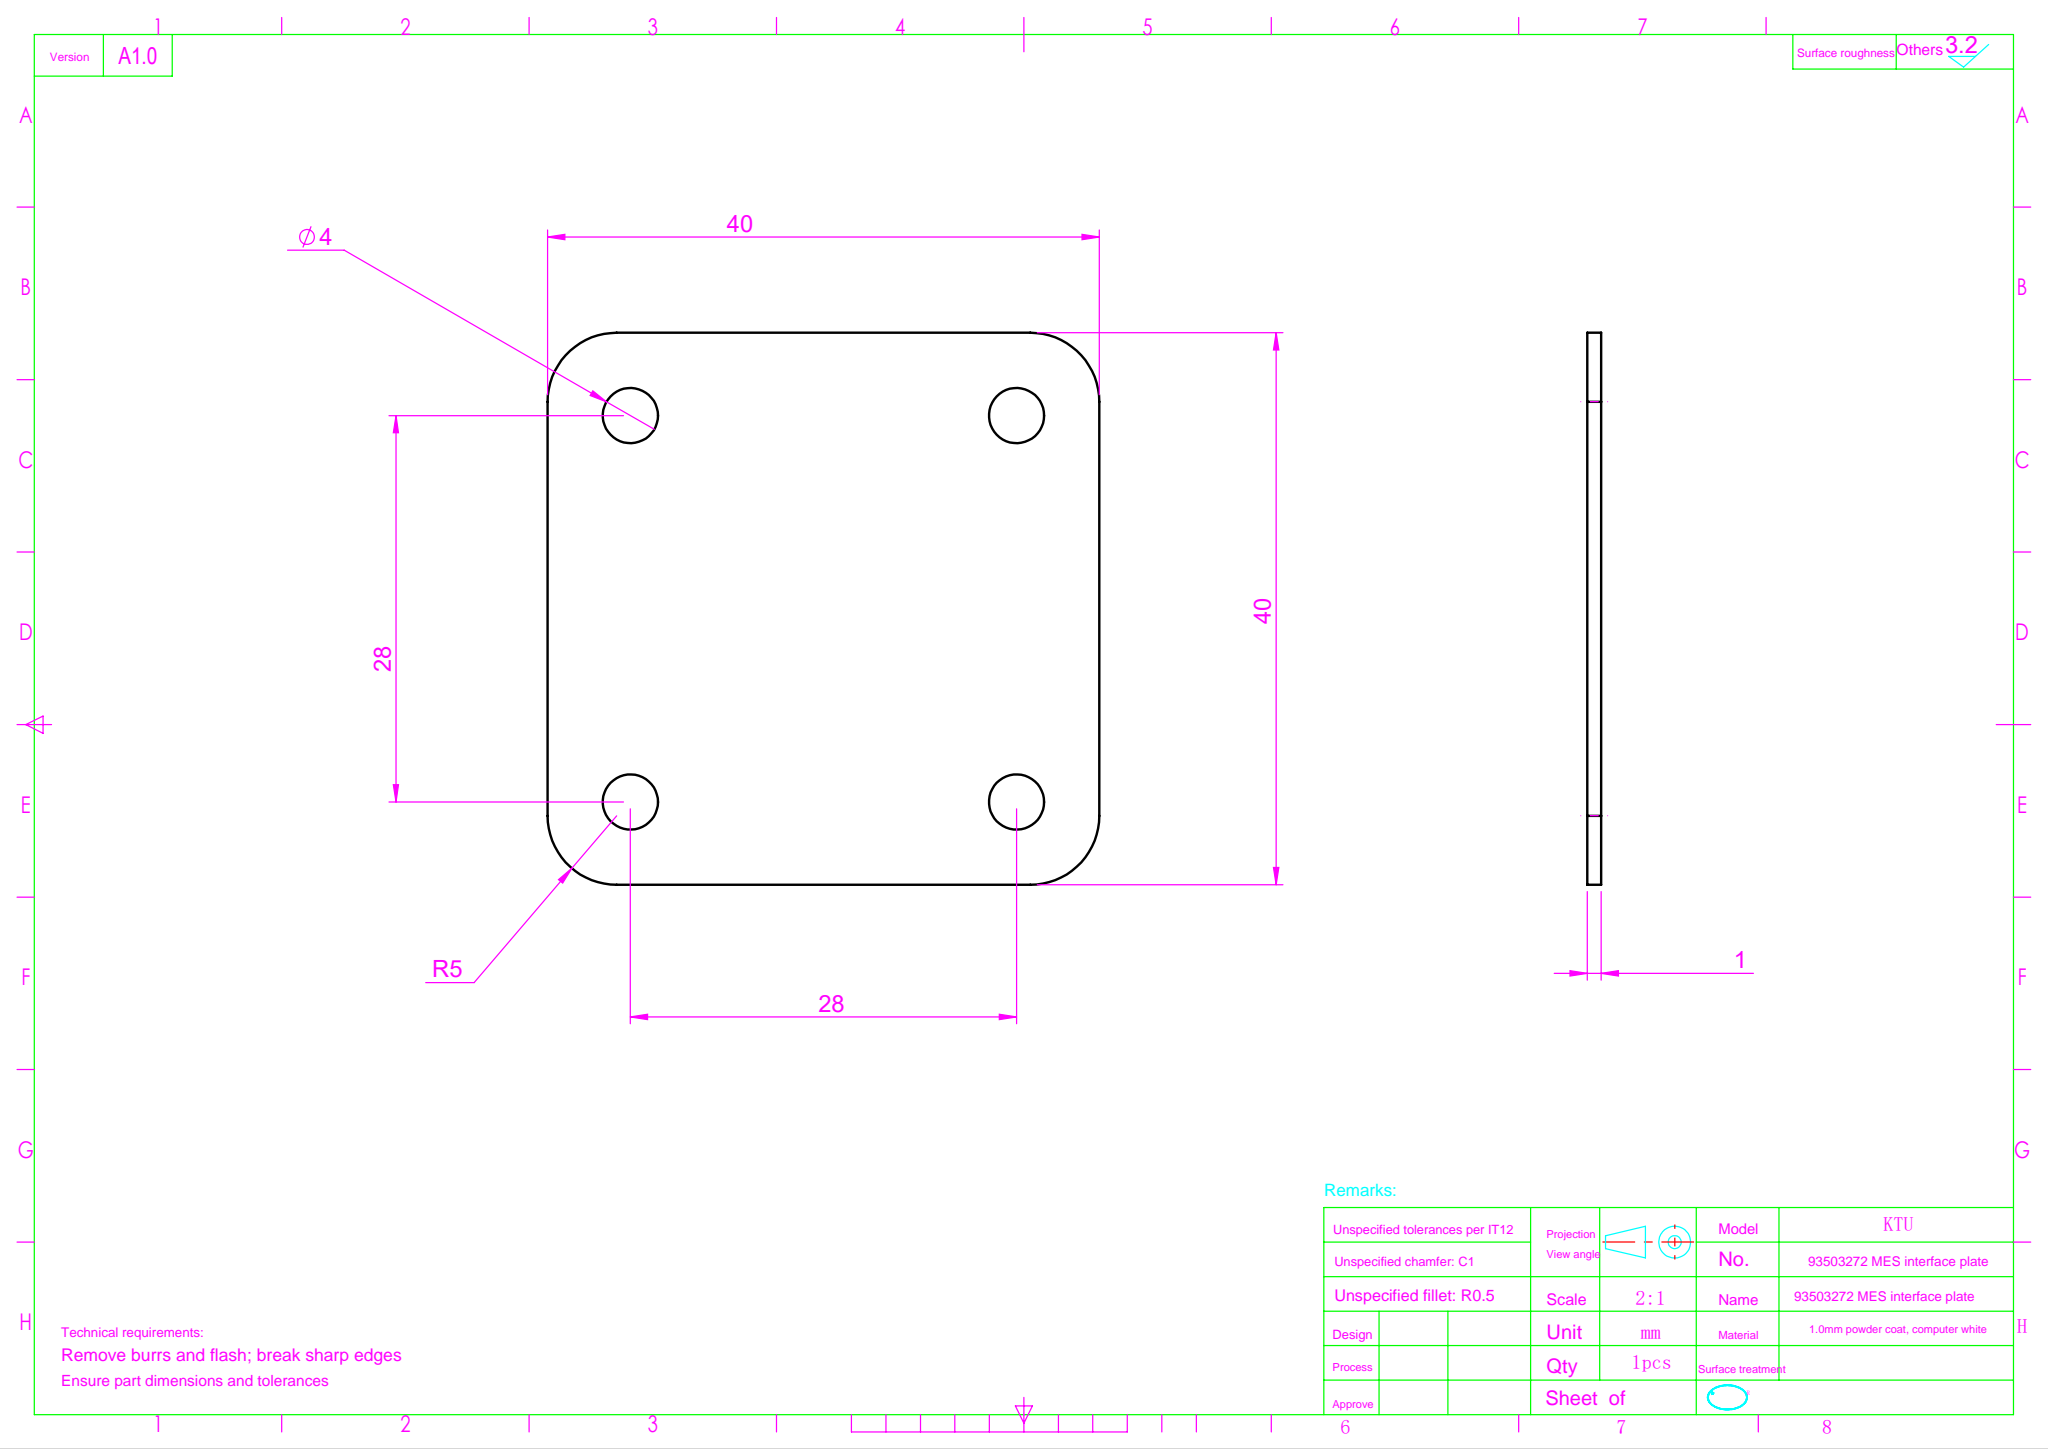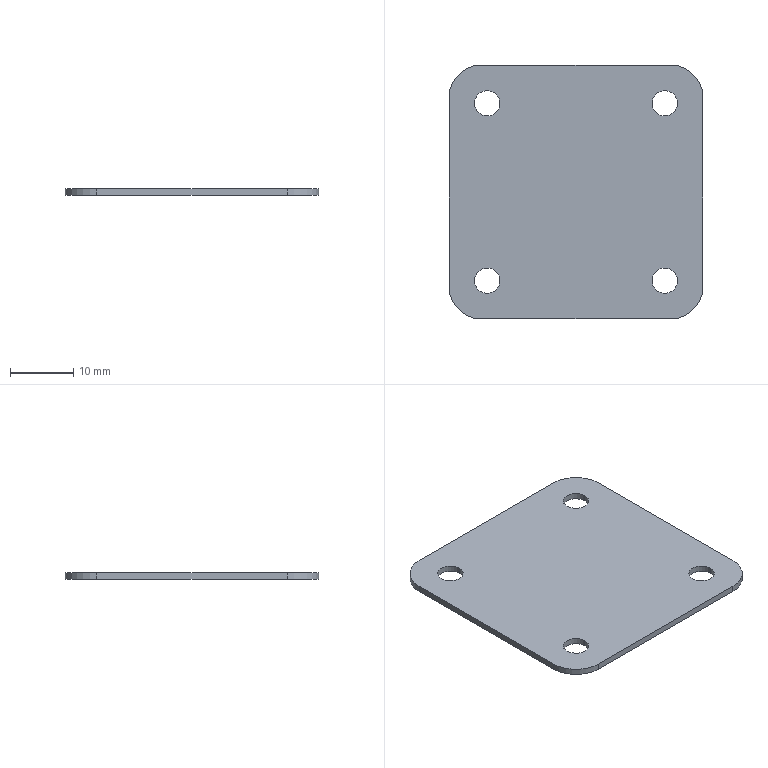Part | SolidWorks | features FlatPattern 1, SMBaseFlange 1, SheetMetal 1 | 1 solid | 18 faces | box 40 x 40 x 1 mm | volume 1528 mm3 | cylinder 12 | plane 6 | commonest cylinder face diameters 4 x8 10 x4
STEP:
#1=CARTESIAN_POINT('',(32.,6.,-1.));
#2=VERTEX_POINT('',#1);
#3=CARTESIAN_POINT('',(36.,6.,-1.));
#4=VERTEX_POINT('',#3);
#5=CARTESIAN_POINT('',(34.,6.,-1.));
#6=DIRECTION('',(0.,0.,1.));
#7=DIRECTION('',(1.,0.,0.));
#8=AXIS2_PLACEMENT_3D('',#5,#6,#7);
#9=CIRCLE('',#8,2.);
#10=EDGE_CURVE('',#2,#4,#9,.T.);
#11=ORIENTED_EDGE('',*,*,#10,.F.);
#12=CARTESIAN_POINT('',(32.,6.,0.));
#13=VERTEX_POINT('',#12);
#14=CARTESIAN_POINT('',(32.,6.,-1.));
#15=DIRECTION('',(0.,0.,1.));
#16=VECTOR('',#15,1000.);
#17=LINE('',#14,#16);
#18=EDGE_CURVE('',#2,#13,#17,.T.);
#19=ORIENTED_EDGE('',*,*,#18,.T.);
#20=CARTESIAN_POINT('',(36.,6.,0.));
#21=VERTEX_POINT('',#20);
#22=CARTESIAN_POINT('',(34.,6.,0.));
#23=DIRECTION('',(0.,0.,1.));
#24=DIRECTION('',(1.,0.,0.));
#25=AXIS2_PLACEMENT_3D('',#22,#23,#24);
#26=CIRCLE('',#25,2.);
#27=EDGE_CURVE('',#13,#21,#26,.T.);
#28=ORIENTED_EDGE('',*,*,#27,.T.);
#29=CARTESIAN_POINT('',(36.,6.,-1.));
#30=DIRECTION('',(0.,0.,1.));
#31=VECTOR('',#30,1000.);
#32=LINE('',#29,#31);
#33=EDGE_CURVE('',#4,#21,#32,.T.);
#34=ORIENTED_EDGE('',*,*,#33,.F.);
#35=EDGE_LOOP('',(#11,#19,#28,#34));
#36=FACE_OUTER_BOUND('',#35,.T.);
#37=CARTESIAN_POINT('',(34.,6.,-1.));
#38=DIRECTION('',(0.,0.,1.));
#39=DIRECTION('',(1.,0.,0.));
#40=AXIS2_PLACEMENT_3D('',#37,#38,#39);
#41=CYLINDRICAL_SURFACE('',#40,2.);
#42=ADVANCED_FACE('',(#36),#41,.F.);
#43=CARTESIAN_POINT('',(4.,6.,-1.));
#44=VERTEX_POINT('',#43);
#45=CARTESIAN_POINT('',(8.,6.,-1.));
#46=VERTEX_POINT('',#45);
#47=CARTESIAN_POINT('',(6.,6.,-1.));
#48=DIRECTION('',(0.,0.,1.));
#49=DIRECTION('',(1.,0.,0.));
#50=AXIS2_PLACEMENT_3D('',#47,#48,#49);
#51=CIRCLE('',#50,2.);
#52=EDGE_CURVE('',#44,#46,#51,.T.);
#53=ORIENTED_EDGE('',*,*,#52,.F.);
#54=CARTESIAN_POINT('',(4.,6.,0.));
#55=VERTEX_POINT('',#54);
#56=CARTESIAN_POINT('',(4.,6.,-1.));
#57=DIRECTION('',(0.,0.,1.));
#58=VECTOR('',#57,1000.);
#59=LINE('',#56,#58);
#60=EDGE_CURVE('',#44,#55,#59,.T.);
#61=ORIENTED_EDGE('',*,*,#60,.T.);
#62=CARTESIAN_POINT('',(8.,6.,0.));
#63=VERTEX_POINT('',#62);
#64=CARTESIAN_POINT('',(6.,6.,0.));
#65=DIRECTION('',(0.,0.,1.));
#66=DIRECTION('',(1.,0.,0.));
#67=AXIS2_PLACEMENT_3D('',#64,#65,#66);
#68=CIRCLE('',#67,2.);
#69=EDGE_CURVE('',#55,#63,#68,.T.);
#70=ORIENTED_EDGE('',*,*,#69,.T.);
#71=CARTESIAN_POINT('',(8.,6.,-1.));
#72=DIRECTION('',(0.,0.,1.));
#73=VECTOR('',#72,1000.);
#74=LINE('',#71,#73);
#75=EDGE_CURVE('',#46,#63,#74,.T.);
#76=ORIENTED_EDGE('',*,*,#75,.F.);
#77=EDGE_LOOP('',(#53,#61,#70,#76));
#78=FACE_OUTER_BOUND('',#77,.T.);
#79=CARTESIAN_POINT('',(6.,6.,-1.));
#80=DIRECTION('',(0.,0.,1.));
#81=DIRECTION('',(1.,0.,0.));
#82=AXIS2_PLACEMENT_3D('',#79,#80,#81);
#83=CYLINDRICAL_SURFACE('',#82,2.);
#84=ADVANCED_FACE('',(#78),#83,.F.);
#85=CARTESIAN_POINT('',(4.,34.,-1.));
#86=VERTEX_POINT('',#85);
#87=CARTESIAN_POINT('',(8.,34.,-1.));
#88=VERTEX_POINT('',#87);
#89=CARTESIAN_POINT('',(6.,34.,-1.));
#90=DIRECTION('',(0.,0.,1.));
#91=DIRECTION('',(1.,0.,0.));
#92=AXIS2_PLACEMENT_3D('',#89,#90,#91);
#93=CIRCLE('',#92,2.);
#94=EDGE_CURVE('',#86,#88,#93,.T.);
#95=ORIENTED_EDGE('',*,*,#94,.F.);
#96=CARTESIAN_POINT('',(4.,34.,0.));
#97=VERTEX_POINT('',#96);
#98=CARTESIAN_POINT('',(4.,34.,-1.));
#99=DIRECTION('',(0.,0.,1.));
#100=VECTOR('',#99,1000.);
#101=LINE('',#98,#100);
#102=EDGE_CURVE('',#86,#97,#101,.T.);
#103=ORIENTED_EDGE('',*,*,#102,.T.);
#104=CARTESIAN_POINT('',(8.,34.,0.));
#105=VERTEX_POINT('',#104);
#106=CARTESIAN_POINT('',(6.,34.,0.));
#107=DIRECTION('',(0.,0.,1.));
#108=DIRECTION('',(1.,0.,0.));
#109=AXIS2_PLACEMENT_3D('',#106,#107,#108);
#110=CIRCLE('',#109,2.);
#111=EDGE_CURVE('',#97,#105,#110,.T.);
#112=ORIENTED_EDGE('',*,*,#111,.T.);
#113=CARTESIAN_POINT('',(8.,34.,-1.));
#114=DIRECTION('',(0.,0.,1.));
#115=VECTOR('',#114,1000.);
#116=LINE('',#113,#115);
#117=EDGE_CURVE('',#88,#105,#116,.T.);
#118=ORIENTED_EDGE('',*,*,#117,.F.);
#119=EDGE_LOOP('',(#95,#103,#112,#118));
#120=FACE_OUTER_BOUND('',#119,.T.);
#121=CARTESIAN_POINT('',(6.,34.,-1.));
#122=DIRECTION('',(0.,0.,1.));
#123=DIRECTION('',(1.,0.,0.));
#124=AXIS2_PLACEMENT_3D('',#121,#122,#123);
#125=CYLINDRICAL_SURFACE('',#124,2.);
#126=ADVANCED_FACE('',(#120),#125,.F.);
#127=CARTESIAN_POINT('',(32.,34.,-1.));
#128=VERTEX_POINT('',#127);
#129=CARTESIAN_POINT('',(36.,34.,-1.));
#130=VERTEX_POINT('',#129);
#131=CARTESIAN_POINT('',(34.,34.,-1.));
#132=DIRECTION('',(0.,0.,1.));
#133=DIRECTION('',(1.,0.,0.));
#134=AXIS2_PLACEMENT_3D('',#131,#132,#133);
#135=CIRCLE('',#134,2.);
#136=EDGE_CURVE('',#128,#130,#135,.T.);
#137=ORIENTED_EDGE('',*,*,#136,.F.);
#138=CARTESIAN_POINT('',(32.,34.,0.));
#139=VERTEX_POINT('',#138);
#140=CARTESIAN_POINT('',(32.,34.,-1.));
#141=DIRECTION('',(0.,0.,1.));
#142=VECTOR('',#141,1000.);
#143=LINE('',#140,#142);
#144=EDGE_CURVE('',#128,#139,#143,.T.);
#145=ORIENTED_EDGE('',*,*,#144,.T.);
#146=CARTESIAN_POINT('',(36.,34.,0.));
#147=VERTEX_POINT('',#146);
#148=CARTESIAN_POINT('',(34.,34.,0.));
#149=DIRECTION('',(0.,0.,1.));
#150=DIRECTION('',(1.,0.,0.));
#151=AXIS2_PLACEMENT_3D('',#148,#149,#150);
#152=CIRCLE('',#151,2.);
#153=EDGE_CURVE('',#139,#147,#152,.T.);
#154=ORIENTED_EDGE('',*,*,#153,.T.);
#155=CARTESIAN_POINT('',(36.,34.,-1.));
#156=DIRECTION('',(0.,0.,1.));
#157=VECTOR('',#156,1000.);
#158=LINE('',#155,#157);
#159=EDGE_CURVE('',#130,#147,#158,.T.);
#160=ORIENTED_EDGE('',*,*,#159,.F.);
#161=EDGE_LOOP('',(#137,#145,#154,#160));
#162=FACE_OUTER_BOUND('',#161,.T.);
#163=CARTESIAN_POINT('',(34.,34.,-1.));
#164=DIRECTION('',(0.,0.,1.));
#165=DIRECTION('',(1.,0.,0.));
#166=AXIS2_PLACEMENT_3D('',#163,#164,#165);
#167=CYLINDRICAL_SURFACE('',#166,2.);
#168=ADVANCED_FACE('',(#162),#167,.F.);
#169=CARTESIAN_POINT('',(40.,35.,0.));
#170=VERTEX_POINT('',#169);
#171=CARTESIAN_POINT('',(35.,40.,0.));
#172=VERTEX_POINT('',#171);
#173=CARTESIAN_POINT('',(35.,35.,0.));
#174=DIRECTION('',(0.,0.,1.));
#175=DIRECTION('',(-1.,0.,0.));
#176=AXIS2_PLACEMENT_3D('',#173,#174,#175);
#177=CIRCLE('',#176,5.);
#178=EDGE_CURVE('',#170,#172,#177,.T.);
#179=ORIENTED_EDGE('',*,*,#178,.F.);
#180=CARTESIAN_POINT('',(40.,35.,-1.));
#181=VERTEX_POINT('',#180);
#182=CARTESIAN_POINT('',(40.,35.,-1.));
#183=DIRECTION('',(0.,0.,1.));
#184=VECTOR('',#183,1000.);
#185=LINE('',#182,#184);
#186=EDGE_CURVE('',#181,#170,#185,.T.);
#187=ORIENTED_EDGE('',*,*,#186,.F.);
#188=CARTESIAN_POINT('',(35.,40.,-1.));
#189=VERTEX_POINT('',#188);
#190=CARTESIAN_POINT('',(35.,35.,-1.));
#191=DIRECTION('',(0.,0.,1.));
#192=DIRECTION('',(-1.,0.,0.));
#193=AXIS2_PLACEMENT_3D('',#190,#191,#192);
#194=CIRCLE('',#193,5.);
#195=EDGE_CURVE('',#181,#189,#194,.T.);
#196=ORIENTED_EDGE('',*,*,#195,.T.);
#197=CARTESIAN_POINT('',(35.,40.,-1.));
#198=DIRECTION('',(0.,0.,1.));
#199=VECTOR('',#198,1000.);
#200=LINE('',#197,#199);
#201=EDGE_CURVE('',#189,#172,#200,.T.);
#202=ORIENTED_EDGE('',*,*,#201,.T.);
#203=EDGE_LOOP('',(#179,#187,#196,#202));
#204=FACE_OUTER_BOUND('',#203,.T.);
#205=CARTESIAN_POINT('',(35.,35.,-1.));
#206=DIRECTION('',(0.,0.,1.));
#207=DIRECTION('',(1.,0.,0.));
#208=AXIS2_PLACEMENT_3D('',#205,#206,#207);
#209=CYLINDRICAL_SURFACE('',#208,5.);
#210=ADVANCED_FACE('',(#204),#209,.T.);
#211=CARTESIAN_POINT('',(40.,5.,0.));
#212=VERTEX_POINT('',#211);
#213=CARTESIAN_POINT('',(40.,5.,0.));
#214=DIRECTION('',(0.,1.,0.));
#215=VECTOR('',#214,1000.);
#216=LINE('',#213,#215);
#217=EDGE_CURVE('',#212,#170,#216,.T.);
#218=ORIENTED_EDGE('',*,*,#217,.F.);
#219=CARTESIAN_POINT('',(40.,5.,-1.));
#220=VERTEX_POINT('',#219);
#221=CARTESIAN_POINT('',(40.,5.,-1.));
#222=DIRECTION('',(0.,0.,1.));
#223=VECTOR('',#222,1000.);
#224=LINE('',#221,#223);
#225=EDGE_CURVE('',#220,#212,#224,.T.);
#226=ORIENTED_EDGE('',*,*,#225,.F.);
#227=CARTESIAN_POINT('',(40.,5.,-1.));
#228=DIRECTION('',(0.,1.,0.));
#229=VECTOR('',#228,1000.);
#230=LINE('',#227,#229);
#231=EDGE_CURVE('',#220,#181,#230,.T.);
#232=ORIENTED_EDGE('',*,*,#231,.T.);
#233=ORIENTED_EDGE('',*,*,#186,.T.);
#234=EDGE_LOOP('',(#218,#226,#232,#233));
#235=FACE_OUTER_BOUND('',#234,.T.);
#236=CARTESIAN_POINT('',(40.,5.,-1.));
#237=DIRECTION('',(1.,0.,0.));
#238=DIRECTION('',(0.,1.,0.));
#239=AXIS2_PLACEMENT_3D('',#236,#237,#238);
#240=PLANE('',#239);
#241=ADVANCED_FACE('',(#235),#240,.T.);
#242=CARTESIAN_POINT('',(35.,0.,0.));
#243=VERTEX_POINT('',#242);
#244=CARTESIAN_POINT('',(35.,5.,0.));
#245=DIRECTION('',(0.,0.,1.));
#246=DIRECTION('',(-1.,0.,0.));
#247=AXIS2_PLACEMENT_3D('',#244,#245,#246);
#248=CIRCLE('',#247,5.);
#249=EDGE_CURVE('',#243,#212,#248,.T.);
#250=ORIENTED_EDGE('',*,*,#249,.F.);
#251=CARTESIAN_POINT('',(35.,0.,-1.));
#252=VERTEX_POINT('',#251);
#253=CARTESIAN_POINT('',(35.,0.,-1.));
#254=DIRECTION('',(0.,0.,1.));
#255=VECTOR('',#254,1000.);
#256=LINE('',#253,#255);
#257=EDGE_CURVE('',#252,#243,#256,.T.);
#258=ORIENTED_EDGE('',*,*,#257,.F.);
#259=CARTESIAN_POINT('',(35.,5.,-1.));
#260=DIRECTION('',(0.,0.,1.));
#261=DIRECTION('',(-1.,0.,0.));
#262=AXIS2_PLACEMENT_3D('',#259,#260,#261);
#263=CIRCLE('',#262,5.);
#264=EDGE_CURVE('',#252,#220,#263,.T.);
#265=ORIENTED_EDGE('',*,*,#264,.T.);
#266=ORIENTED_EDGE('',*,*,#225,.T.);
#267=EDGE_LOOP('',(#250,#258,#265,#266));
#268=FACE_OUTER_BOUND('',#267,.T.);
#269=CARTESIAN_POINT('',(35.,5.,-1.));
#270=DIRECTION('',(0.,0.,1.));
#271=DIRECTION('',(1.,0.,0.));
#272=AXIS2_PLACEMENT_3D('',#269,#270,#271);
#273=CYLINDRICAL_SURFACE('',#272,5.);
#274=ADVANCED_FACE('',(#268),#273,.T.);
#275=CARTESIAN_POINT('',(5.,0.,0.));
#276=VERTEX_POINT('',#275);
#277=CARTESIAN_POINT('',(5.,0.,0.));
#278=DIRECTION('',(1.,0.,0.));
#279=VECTOR('',#278,1000.);
#280=LINE('',#277,#279);
#281=EDGE_CURVE('',#276,#243,#280,.T.);
#282=ORIENTED_EDGE('',*,*,#281,.F.);
#283=CARTESIAN_POINT('',(5.,0.,-1.));
#284=VERTEX_POINT('',#283);
#285=CARTESIAN_POINT('',(5.,0.,-1.));
#286=DIRECTION('',(0.,0.,1.));
#287=VECTOR('',#286,1000.);
#288=LINE('',#285,#287);
#289=EDGE_CURVE('',#284,#276,#288,.T.);
#290=ORIENTED_EDGE('',*,*,#289,.F.);
#291=CARTESIAN_POINT('',(5.,0.,-1.));
#292=DIRECTION('',(1.,0.,0.));
#293=VECTOR('',#292,1000.);
#294=LINE('',#291,#293);
#295=EDGE_CURVE('',#284,#252,#294,.T.);
#296=ORIENTED_EDGE('',*,*,#295,.T.);
#297=ORIENTED_EDGE('',*,*,#257,.T.);
#298=EDGE_LOOP('',(#282,#290,#296,#297));
#299=FACE_OUTER_BOUND('',#298,.T.);
#300=CARTESIAN_POINT('',(5.,0.,-1.));
#301=DIRECTION('',(0.,-1.,0.));
#302=DIRECTION('',(0.,0.,-1.));
#303=AXIS2_PLACEMENT_3D('',#300,#301,#302);
#304=PLANE('',#303);
#305=ADVANCED_FACE('',(#299),#304,.T.);
#306=CARTESIAN_POINT('',(0.,5.,0.));
#307=VERTEX_POINT('',#306);
#308=CARTESIAN_POINT('',(5.,5.,0.));
#309=DIRECTION('',(0.,0.,1.));
#310=DIRECTION('',(-1.,0.,0.));
#311=AXIS2_PLACEMENT_3D('',#308,#309,#310);
#312=CIRCLE('',#311,5.);
#313=EDGE_CURVE('',#307,#276,#312,.T.);
#314=ORIENTED_EDGE('',*,*,#313,.F.);
#315=CARTESIAN_POINT('',(0.,5.,-1.));
#316=VERTEX_POINT('',#315);
#317=CARTESIAN_POINT('',(0.,5.,-1.));
#318=DIRECTION('',(0.,0.,1.));
#319=VECTOR('',#318,1000.);
#320=LINE('',#317,#319);
#321=EDGE_CURVE('',#316,#307,#320,.T.);
#322=ORIENTED_EDGE('',*,*,#321,.F.);
#323=CARTESIAN_POINT('',(5.,5.,-1.));
#324=DIRECTION('',(0.,0.,1.));
#325=DIRECTION('',(-1.,0.,0.));
#326=AXIS2_PLACEMENT_3D('',#323,#324,#325);
#327=CIRCLE('',#326,5.);
#328=EDGE_CURVE('',#316,#284,#327,.T.);
#329=ORIENTED_EDGE('',*,*,#328,.T.);
#330=ORIENTED_EDGE('',*,*,#289,.T.);
#331=EDGE_LOOP('',(#314,#322,#329,#330));
#332=FACE_OUTER_BOUND('',#331,.T.);
#333=CARTESIAN_POINT('',(5.,5.,-1.));
#334=DIRECTION('',(0.,0.,1.));
#335=DIRECTION('',(1.,0.,0.));
#336=AXIS2_PLACEMENT_3D('',#333,#334,#335);
#337=CYLINDRICAL_SURFACE('',#336,5.);
#338=ADVANCED_FACE('',(#332),#337,.T.);
#339=CARTESIAN_POINT('',(0.,35.,0.));
#340=VERTEX_POINT('',#339);
#341=CARTESIAN_POINT('',(0.,5.,0.));
#342=DIRECTION('',(0.,-1.,0.));
#343=VECTOR('',#342,1000.);
#344=LINE('',#341,#343);
#345=EDGE_CURVE('',#340,#307,#344,.T.);
#346=ORIENTED_EDGE('',*,*,#345,.F.);
#347=CARTESIAN_POINT('',(0.,35.,-1.));
#348=VERTEX_POINT('',#347);
#349=CARTESIAN_POINT('',(0.,35.,-1.));
#350=DIRECTION('',(0.,0.,1.));
#351=VECTOR('',#350,1000.);
#352=LINE('',#349,#351);
#353=EDGE_CURVE('',#348,#340,#352,.T.);
#354=ORIENTED_EDGE('',*,*,#353,.F.);
#355=CARTESIAN_POINT('',(0.,5.,-1.));
#356=DIRECTION('',(0.,-1.,0.));
#357=VECTOR('',#356,1000.);
#358=LINE('',#355,#357);
#359=EDGE_CURVE('',#348,#316,#358,.T.);
#360=ORIENTED_EDGE('',*,*,#359,.T.);
#361=ORIENTED_EDGE('',*,*,#321,.T.);
#362=EDGE_LOOP('',(#346,#354,#360,#361));
#363=FACE_OUTER_BOUND('',#362,.T.);
#364=CARTESIAN_POINT('',(0.,5.,-1.));
#365=DIRECTION('',(-1.,0.,0.));
#366=DIRECTION('',(0.,-1.,0.));
#367=AXIS2_PLACEMENT_3D('',#364,#365,#366);
#368=PLANE('',#367);
#369=ADVANCED_FACE('',(#363),#368,.T.);
#370=CARTESIAN_POINT('',(5.,40.,0.));
#371=VERTEX_POINT('',#370);
#372=CARTESIAN_POINT('',(5.,35.,0.));
#373=DIRECTION('',(0.,0.,1.));
#374=DIRECTION('',(-1.,0.,0.));
#375=AXIS2_PLACEMENT_3D('',#372,#373,#374);
#376=CIRCLE('',#375,5.);
#377=EDGE_CURVE('',#371,#340,#376,.T.);
#378=ORIENTED_EDGE('',*,*,#377,.F.);
#379=CARTESIAN_POINT('',(5.,40.,-1.));
#380=VERTEX_POINT('',#379);
#381=CARTESIAN_POINT('',(5.,40.,-1.));
#382=DIRECTION('',(0.,0.,1.));
#383=VECTOR('',#382,1000.);
#384=LINE('',#381,#383);
#385=EDGE_CURVE('',#380,#371,#384,.T.);
#386=ORIENTED_EDGE('',*,*,#385,.F.);
#387=CARTESIAN_POINT('',(5.,35.,-1.));
#388=DIRECTION('',(0.,0.,1.));
#389=DIRECTION('',(-1.,0.,0.));
#390=AXIS2_PLACEMENT_3D('',#387,#388,#389);
#391=CIRCLE('',#390,5.);
#392=EDGE_CURVE('',#380,#348,#391,.T.);
#393=ORIENTED_EDGE('',*,*,#392,.T.);
#394=ORIENTED_EDGE('',*,*,#353,.T.);
#395=EDGE_LOOP('',(#378,#386,#393,#394));
#396=FACE_OUTER_BOUND('',#395,.T.);
#397=CARTESIAN_POINT('',(5.,35.,-1.));
#398=DIRECTION('',(0.,0.,1.));
#399=DIRECTION('',(1.,0.,0.));
#400=AXIS2_PLACEMENT_3D('',#397,#398,#399);
#401=CYLINDRICAL_SURFACE('',#400,5.);
#402=ADVANCED_FACE('',(#396),#401,.T.);
#403=CARTESIAN_POINT('',(5.,40.,0.));
#404=DIRECTION('',(-1.,0.,0.));
#405=VECTOR('',#404,1000.);
#406=LINE('',#403,#405);
#407=EDGE_CURVE('',#172,#371,#406,.T.);
#408=ORIENTED_EDGE('',*,*,#407,.F.);
#409=ORIENTED_EDGE('',*,*,#201,.F.);
#410=CARTESIAN_POINT('',(5.,40.,-1.));
#411=DIRECTION('',(-1.,0.,0.));
#412=VECTOR('',#411,1000.);
#413=LINE('',#410,#412);
#414=EDGE_CURVE('',#189,#380,#413,.T.);
#415=ORIENTED_EDGE('',*,*,#414,.T.);
#416=ORIENTED_EDGE('',*,*,#385,.T.);
#417=EDGE_LOOP('',(#408,#409,#415,#416));
#418=FACE_OUTER_BOUND('',#417,.T.);
#419=CARTESIAN_POINT('',(5.,40.,-1.));
#420=DIRECTION('',(0.,1.,0.));
#421=DIRECTION('',(0.,0.,1.));
#422=AXIS2_PLACEMENT_3D('',#419,#420,#421);
#423=PLANE('',#422);
#424=ADVANCED_FACE('',(#418),#423,.T.);
#425=CARTESIAN_POINT('',(34.,6.,-1.));
#426=DIRECTION('',(0.,0.,1.));
#427=DIRECTION('',(1.,0.,0.));
#428=AXIS2_PLACEMENT_3D('',#425,#426,#427);
#429=CIRCLE('',#428,2.);
#430=EDGE_CURVE('',#4,#2,#429,.T.);
#431=ORIENTED_EDGE('',*,*,#430,.T.);
#432=ORIENTED_EDGE('',*,*,#10,.T.);
#433=EDGE_LOOP('',(#431,#432));
#434=FACE_BOUND('',#433,.T.);
#435=CARTESIAN_POINT('',(6.,6.,-1.));
#436=DIRECTION('',(0.,0.,1.));
#437=DIRECTION('',(1.,0.,0.));
#438=AXIS2_PLACEMENT_3D('',#435,#436,#437);
#439=CIRCLE('',#438,2.);
#440=EDGE_CURVE('',#46,#44,#439,.T.);
#441=ORIENTED_EDGE('',*,*,#440,.T.);
#442=ORIENTED_EDGE('',*,*,#52,.T.);
#443=EDGE_LOOP('',(#441,#442));
#444=FACE_BOUND('',#443,.T.);
#445=CARTESIAN_POINT('',(6.,34.,-1.));
#446=DIRECTION('',(0.,0.,1.));
#447=DIRECTION('',(1.,0.,0.));
#448=AXIS2_PLACEMENT_3D('',#445,#446,#447);
#449=CIRCLE('',#448,2.);
#450=EDGE_CURVE('',#88,#86,#449,.T.);
#451=ORIENTED_EDGE('',*,*,#450,.T.);
#452=ORIENTED_EDGE('',*,*,#94,.T.);
#453=EDGE_LOOP('',(#451,#452));
#454=FACE_BOUND('',#453,.T.);
#455=CARTESIAN_POINT('',(34.,34.,-1.));
#456=DIRECTION('',(0.,0.,1.));
#457=DIRECTION('',(1.,0.,0.));
#458=AXIS2_PLACEMENT_3D('',#455,#456,#457);
#459=CIRCLE('',#458,2.);
#460=EDGE_CURVE('',#130,#128,#459,.T.);
#461=ORIENTED_EDGE('',*,*,#460,.T.);
#462=ORIENTED_EDGE('',*,*,#136,.T.);
#463=EDGE_LOOP('',(#461,#462));
#464=FACE_BOUND('',#463,.T.);
#465=ORIENTED_EDGE('',*,*,#195,.F.);
#466=ORIENTED_EDGE('',*,*,#231,.F.);
#467=ORIENTED_EDGE('',*,*,#264,.F.);
#468=ORIENTED_EDGE('',*,*,#295,.F.);
#469=ORIENTED_EDGE('',*,*,#328,.F.);
#470=ORIENTED_EDGE('',*,*,#359,.F.);
#471=ORIENTED_EDGE('',*,*,#392,.F.);
#472=ORIENTED_EDGE('',*,*,#414,.F.);
#473=EDGE_LOOP('',(#465,#466,#467,#468,#469,#470,#471,#472));
#474=FACE_OUTER_BOUND('',#473,.T.);
#475=CARTESIAN_POINT('',(35.,35.,-1.));
#476=DIRECTION('',(0.,0.,-1.));
#477=DIRECTION('',(-1.,0.,0.));
#478=AXIS2_PLACEMENT_3D('',#475,#476,#477);
#479=PLANE('',#478);
#480=ADVANCED_FACE('',(#434,#444,#454,#464,#474),#479,.T.);
#481=CARTESIAN_POINT('',(34.,6.,0.));
#482=DIRECTION('',(0.,0.,1.));
#483=DIRECTION('',(1.,0.,0.));
#484=AXIS2_PLACEMENT_3D('',#481,#482,#483);
#485=CIRCLE('',#484,2.);
#486=EDGE_CURVE('',#21,#13,#485,.T.);
#487=ORIENTED_EDGE('',*,*,#486,.F.);
#488=ORIENTED_EDGE('',*,*,#27,.F.);
#489=EDGE_LOOP('',(#487,#488));
#490=FACE_BOUND('',#489,.T.);
#491=CARTESIAN_POINT('',(6.,6.,0.));
#492=DIRECTION('',(0.,0.,1.));
#493=DIRECTION('',(1.,0.,0.));
#494=AXIS2_PLACEMENT_3D('',#491,#492,#493);
#495=CIRCLE('',#494,2.);
#496=EDGE_CURVE('',#63,#55,#495,.T.);
#497=ORIENTED_EDGE('',*,*,#496,.F.);
#498=ORIENTED_EDGE('',*,*,#69,.F.);
#499=EDGE_LOOP('',(#497,#498));
#500=FACE_BOUND('',#499,.T.);
#501=CARTESIAN_POINT('',(6.,34.,0.));
#502=DIRECTION('',(0.,0.,1.));
#503=DIRECTION('',(1.,0.,0.));
#504=AXIS2_PLACEMENT_3D('',#501,#502,#503);
#505=CIRCLE('',#504,2.);
#506=EDGE_CURVE('',#105,#97,#505,.T.);
#507=ORIENTED_EDGE('',*,*,#506,.F.);
#508=ORIENTED_EDGE('',*,*,#111,.F.);
#509=EDGE_LOOP('',(#507,#508));
#510=FACE_BOUND('',#509,.T.);
#511=CARTESIAN_POINT('',(34.,34.,0.));
#512=DIRECTION('',(0.,0.,1.));
#513=DIRECTION('',(1.,0.,0.));
#514=AXIS2_PLACEMENT_3D('',#511,#512,#513);
#515=CIRCLE('',#514,2.);
#516=EDGE_CURVE('',#147,#139,#515,.T.);
#517=ORIENTED_EDGE('',*,*,#516,.F.);
#518=ORIENTED_EDGE('',*,*,#153,.F.);
#519=EDGE_LOOP('',(#517,#518));
#520=FACE_BOUND('',#519,.T.);
#521=ORIENTED_EDGE('',*,*,#178,.T.);
#522=ORIENTED_EDGE('',*,*,#407,.T.);
#523=ORIENTED_EDGE('',*,*,#377,.T.);
#524=ORIENTED_EDGE('',*,*,#345,.T.);
#525=ORIENTED_EDGE('',*,*,#313,.T.);
#526=ORIENTED_EDGE('',*,*,#281,.T.);
#527=ORIENTED_EDGE('',*,*,#249,.T.);
#528=ORIENTED_EDGE('',*,*,#217,.T.);
#529=EDGE_LOOP('',(#521,#522,#523,#524,#525,#526,#527,#528));
#530=FACE_OUTER_BOUND('',#529,.T.);
#531=CARTESIAN_POINT('',(35.,35.,0.));
#532=DIRECTION('',(0.,0.,-1.));
#533=DIRECTION('',(-1.,0.,0.));
#534=AXIS2_PLACEMENT_3D('',#531,#532,#533);
#535=PLANE('',#534);
#536=ADVANCED_FACE('',(#490,#500,#510,#520,#530),#535,.F.);
#537=ORIENTED_EDGE('',*,*,#144,.F.);
#538=ORIENTED_EDGE('',*,*,#460,.F.);
#539=ORIENTED_EDGE('',*,*,#159,.T.);
#540=ORIENTED_EDGE('',*,*,#516,.T.);
#541=EDGE_LOOP('',(#537,#538,#539,#540));
#542=FACE_OUTER_BOUND('',#541,.T.);
#543=CARTESIAN_POINT('',(34.,34.,-1.));
#544=DIRECTION('',(0.,0.,1.));
#545=DIRECTION('',(1.,0.,0.));
#546=AXIS2_PLACEMENT_3D('',#543,#544,#545);
#547=CYLINDRICAL_SURFACE('',#546,2.);
#548=ADVANCED_FACE('',(#542),#547,.F.);
#549=ORIENTED_EDGE('',*,*,#102,.F.);
#550=ORIENTED_EDGE('',*,*,#450,.F.);
#551=ORIENTED_EDGE('',*,*,#117,.T.);
#552=ORIENTED_EDGE('',*,*,#506,.T.);
#553=EDGE_LOOP('',(#549,#550,#551,#552));
#554=FACE_OUTER_BOUND('',#553,.T.);
#555=CARTESIAN_POINT('',(6.,34.,-1.));
#556=DIRECTION('',(0.,0.,1.));
#557=DIRECTION('',(1.,0.,0.));
#558=AXIS2_PLACEMENT_3D('',#555,#556,#557);
#559=CYLINDRICAL_SURFACE('',#558,2.);
#560=ADVANCED_FACE('',(#554),#559,.F.);
#561=ORIENTED_EDGE('',*,*,#60,.F.);
#562=ORIENTED_EDGE('',*,*,#440,.F.);
#563=ORIENTED_EDGE('',*,*,#75,.T.);
#564=ORIENTED_EDGE('',*,*,#496,.T.);
#565=EDGE_LOOP('',(#561,#562,#563,#564));
#566=FACE_OUTER_BOUND('',#565,.T.);
#567=CARTESIAN_POINT('',(6.,6.,-1.));
#568=DIRECTION('',(0.,0.,1.));
#569=DIRECTION('',(1.,0.,0.));
#570=AXIS2_PLACEMENT_3D('',#567,#568,#569);
#571=CYLINDRICAL_SURFACE('',#570,2.);
#572=ADVANCED_FACE('',(#566),#571,.F.);
#573=ORIENTED_EDGE('',*,*,#18,.F.);
#574=ORIENTED_EDGE('',*,*,#430,.F.);
#575=ORIENTED_EDGE('',*,*,#33,.T.);
#576=ORIENTED_EDGE('',*,*,#486,.T.);
#577=EDGE_LOOP('',(#573,#574,#575,#576));
#578=FACE_OUTER_BOUND('',#577,.T.);
#579=CARTESIAN_POINT('',(34.,6.,-1.));
#580=DIRECTION('',(0.,0.,1.));
#581=DIRECTION('',(1.,0.,0.));
#582=AXIS2_PLACEMENT_3D('',#579,#580,#581);
#583=CYLINDRICAL_SURFACE('',#582,2.);
#584=ADVANCED_FACE('',(#578),#583,.F.);
#585=CLOSED_SHELL('',(#42,#84,#126,#168,#210,#241,#274,#305,#338,#369,#402,#424,#480,#536,#548,#560,#572,#584));
#586=MANIFOLD_SOLID_BREP('',#585);
#587=CARTESIAN_POINT('',(0.,0.,0.));
#588=DIRECTION('',(0.,0.,1.));
#589=DIRECTION('',(1.,0.,0.));
#590=AXIS2_PLACEMENT_3D('',#587,#588,#589);
#591=(LENGTH_UNIT()NAMED_UNIT(*)SI_UNIT(.MILLI.,.METRE.));
#592=UNCERTAINTY_MEASURE_WITH_UNIT(LENGTH_MEASURE(0.00001),#591,'','');
#593=(NAMED_UNIT(*)PLANE_ANGLE_UNIT()SI_UNIT($,.RADIAN.));
#594=(NAMED_UNIT(*)SI_UNIT($,.STERADIAN.)SOLID_ANGLE_UNIT());
#595=(GEOMETRIC_REPRESENTATION_CONTEXT(3)GLOBAL_UNCERTAINTY_ASSIGNED_CONTEXT((#592))GLOBAL_UNIT_ASSIGNED_CONTEXT((#591,#593,#594))REPRESENTATION_CONTEXT('',''));
#596=ADVANCED_BREP_SHAPE_REPRESENTATION('',(#586,#590),#595);